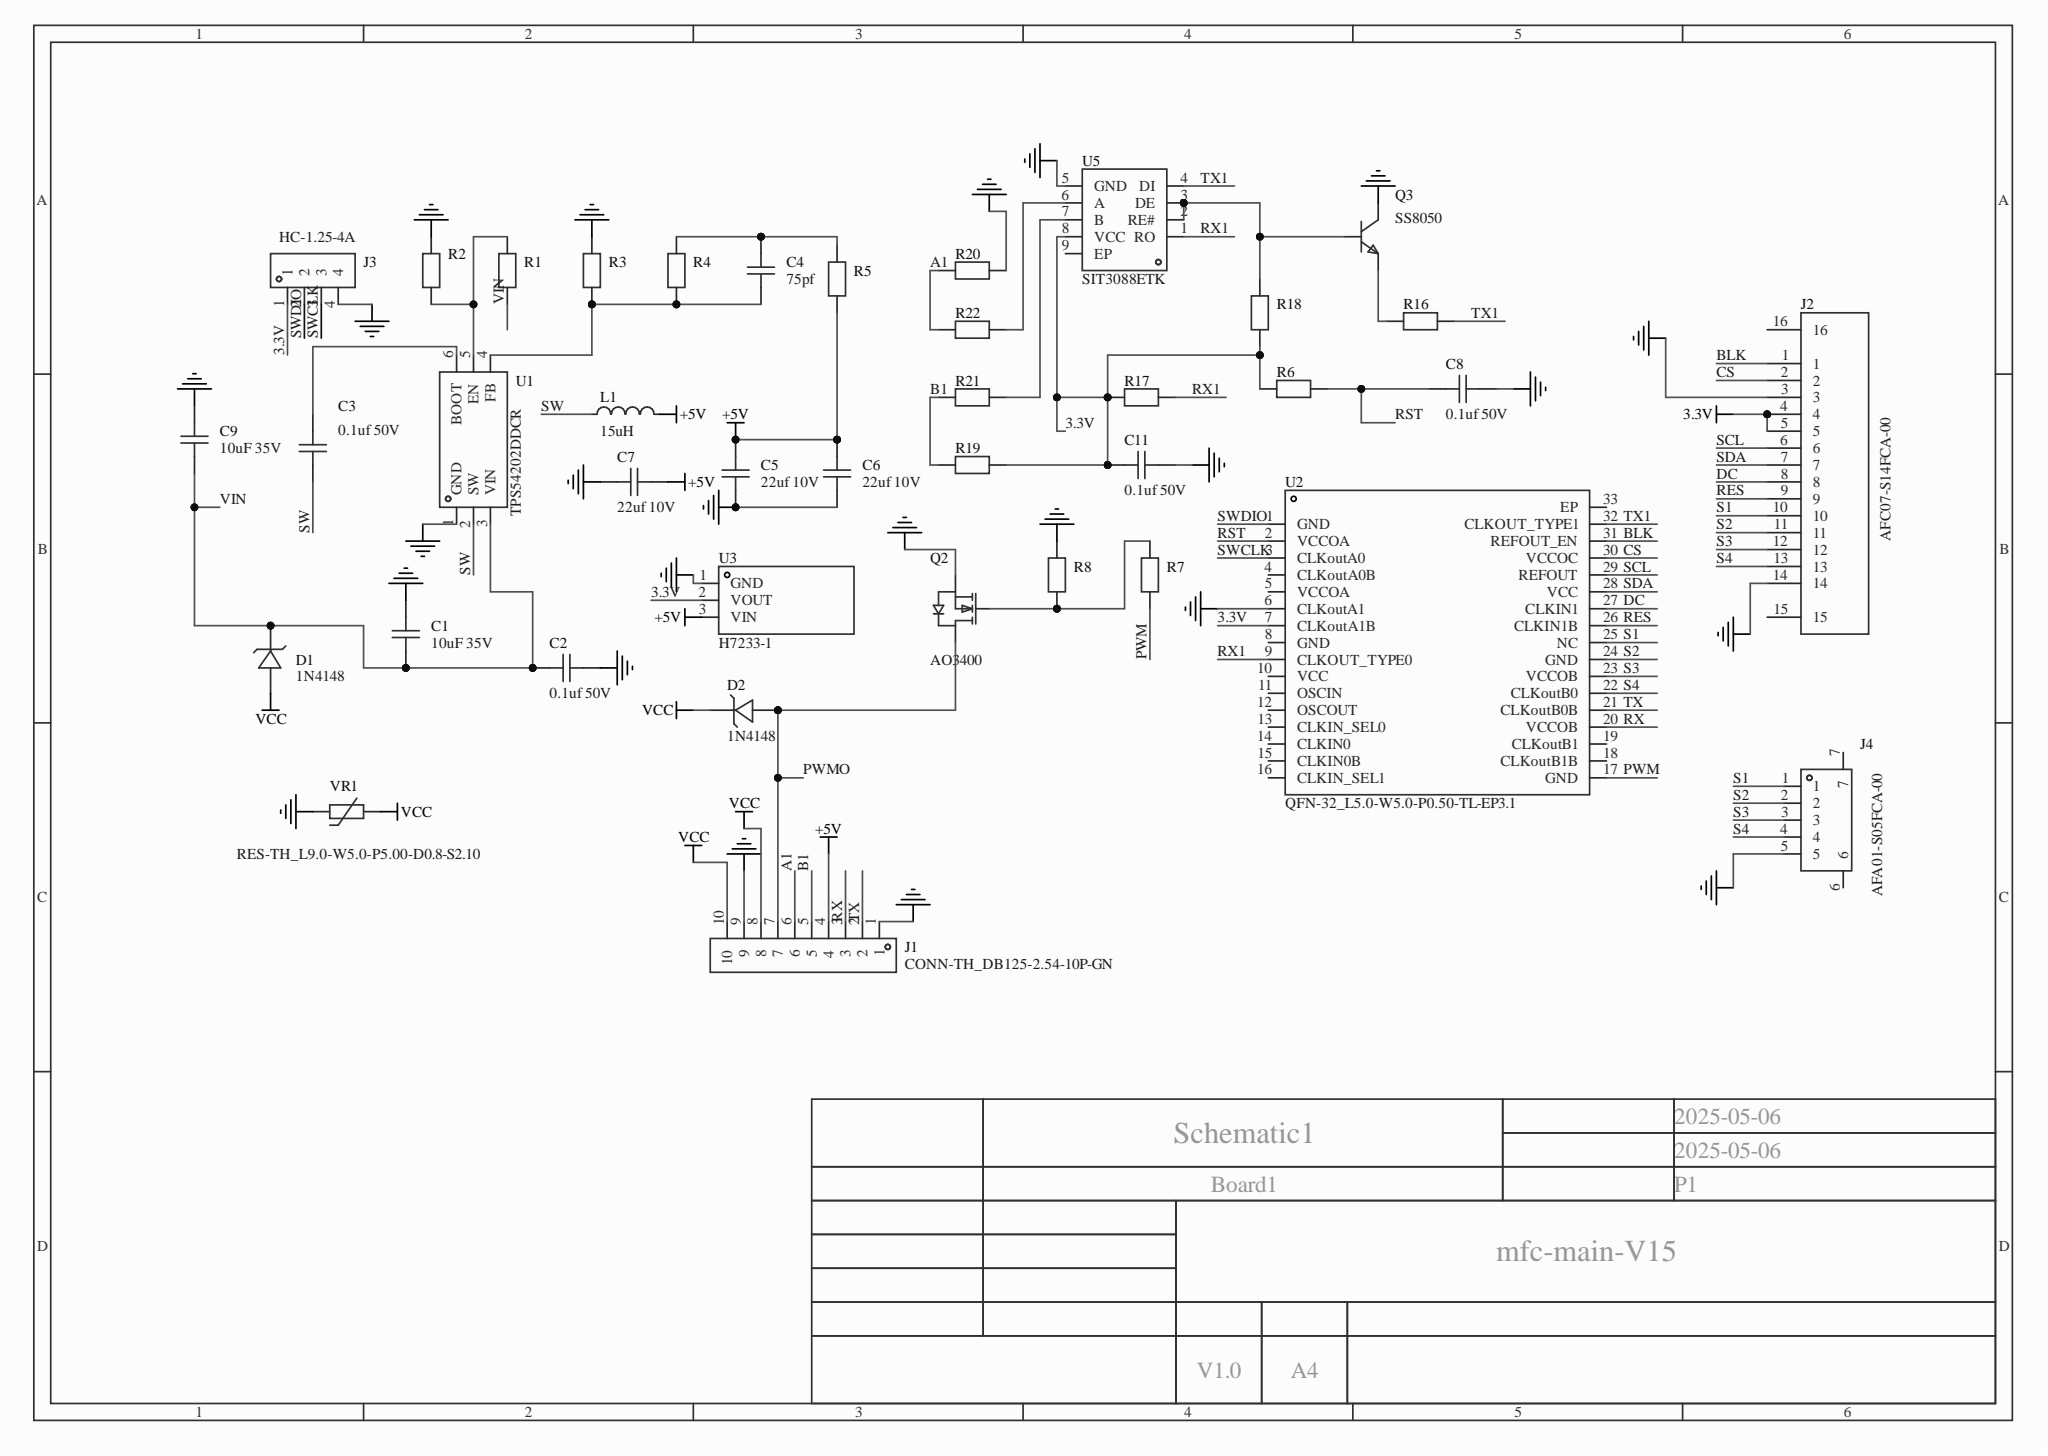Circuit board | Altium Designer | 39 parts | 36 nets
Bill of materials:
Comment,Description,Designator,Footprint,LibRef,Quantity
"10uF 35V","","C1, C9","C0805","CL21A106KAYNNNE_C15850","2"
"0.1uf 50V","","C2, C3, C8, C11","C0603","CT41-0603-2F4-50V-0.1uF-M(N)","4"
"75pf","","C4","C0603","CT41-0603-2F4-50V-0.1uF-M(N)","1"
"22uf 10V","","C5, C6, C7","C0603","CT41-0603-2F4-50V-0.1uF-M(N)","3"
"1N4148","","D1, D2","SOD-123_L2.7-W1.7-LS3.8-RD","1N4148","2"
"CONN-TH_DB125-2.54-10P-GN","","J1","CONN-TH_DB125-2.54-10P-GN","DB125-2.54-10P-GN-S","1"
"AFC07-S14FCA-00","","J2","FPC-SMD_14P-P0.50_AFC07-S14FCA-00","AFC07-S14FCA-00","1"
"HC-1.25-4A","","J3","CONN-TH_4P-P1.25_HCTL_HC-1.25-4A","HC-1.25-4A","1"
"AFA01-S05FCA-00","","J4","FPC-SMD_AFA01-S05FCA-00","AFA01-S05FCA-00","1"
"15uH","","L1","IND-SMD_L3.5-W3.0","CMLF0302-150MTT","1"
"AO3400","","Q2","SOT-23-3_L2.9-W1.3-P1.90-LS2.4-BL-2","AO3400","1"
"SS8050","","Q3","SOT-23-3_L2.9-W1.3-P1.90-LS2.4-BR","SS8050","1"
"","","R1, R2, R3, R4, R5, R6, R7, R8, R16, R17, R18, R19, R20, R21, R22","R0603","RT0603BRD07105KL","15"
"TPS54202DDCR","","U1","SOT-23-6_L2.9-W1.6-P0.95-LS2.8-BL","TPS54202DDCR","1"
"QFN-32_L5.0-W5.0-P0.50-TL-EP3.1","","U2","QFN-32_L5.0-W5.0-P0.50-TL-EP3.1","NCS25D34","1"
"H7233-1","","U3","SOT-23-3_L2.9-W1.3-P1.90-LS2.4-BR","H7233-1","1"
"SIT3088ETK","","U5","DFN-8_L3.0-W3.0-P0.65-BL-EP","SIT3088ETK","1"
"RES-TH_L9.0-W5.0-P5.00-D0.8-S2.10","","VR1","RES-TH_L9.0-W5.0-P5.00-D0.8-S2.10","FTR07D390K","1"
Netlist (Protel format):
[
C1
C0805
10uF 35V



]
[
C2
C0603
0.1uf 50V



]
[
C3
C0603
0.1uf 50V



]
[
C4
C0603
75pf



]
[
C5
C0603
22uf 10V



]
[
C6
C0603
22uf 10V



]
[
C7
C0603
22uf 10V



]
[
C8
C0603
0.1uf 50V



]
[
C9
C0805
10uF 35V



]
[
C11
C0603
0.1uf 50V



]
[
D1
SOD-123_L2.7-W1.7-LS3.8-RD
1N4148



]
[
D2
SOD-123_L2.7-W1.7-LS3.8-RD
1N4148



]
[
J1
CONN-TH_DB125-2.54-10P-GN
CONN-TH_DB125-2.54-10P-GN



]
[
J2
FPC-SMD_14P-P0.50_AFC07-S14FCA-00
AFC07-S14FCA-00



]
[
J3
CONN-TH_4P-P1.25_HCTL_HC-1.25-4A
HC-1.25-4A



]
[
J4
FPC-SMD_AFA01-S05FCA-00
AFA01-S05FCA-00



]
[
L1
IND-SMD_L3.5-W3.0
15uH



]
[
Q2
SOT-23-3_L2.9-W1.3-P1.90-LS2.4-BL-2
AO3400



]
[
Q3
SOT-23-3_L2.9-W1.3-P1.90-LS2.4-BR
SS8050



]
[
R1
R0603




]
[
R2
R0603




]
[
R3
R0603




]
[
R4
R0603




]
[
R5
R0603




]
[
R6
R0603




]
[
R7
R0603




]
[
R8
R0603




]
[
R16
R0603




]
[
R17
R0603




]
[
R18
R0603




]
[
R19
R0603




]
[
R20
R0603




]
[
R21
R0603




]
[
R22
R0603




]
[
U1
SOT-23-6_L2.9-W1.6-P0.95-LS2.8-BL
TPS54202DDCR



]
[
U2
QFN-32_L5.0-W5.0-P0.50-TL-EP3.1
QFN-32_L5.0-W5.0-P0.50-TL-EP3.1



]
[
U3
SOT-23-3_L2.9-W1.3-P1.90-LS2.4-BR
H7233-1



]
[
U5
DFN-8_L3.0-W3.0-P0.65-BL-EP
SIT3088ETK



]
[
VR1
RES-TH_L9.0-W5.0-P5.00-D0.8-S2.10
RES-TH_L9.0-W5.0-P5.00-D0.8-S2.10



]
(
VIN
C1-1
C2-2
C9-1
D1-1
R1-1
U1-3
)
(
VCC
D1-2
D2-1
J1-8
J1-10
VR1-2
)
(
TX1
R16-2
U2-32
U5-4
)
(
TX
J1-2
U2-21
)
(
SWDIO
J3-2
U2-1
)
(
SWCLK
J3-3
U2-3
)
(
SW
C3-1
L1-1
U1-2
)
(
SDA
J2-7
U2-28
)
(
SCL
J2-6
U2-29
)
(
S4
J2-13
J4-4
U2-22
)
(
S3
J2-12
J4-3
U2-23
)
(
S2
J2-11
J4-2
U2-24
)
(
S1
J2-10
J4-1
U2-25
)
(
RX1
R17-2
U2-9
U5-1
)
(
RX
J1-3
U2-20
)
(
RST
C8-2
R6-2
U2-2
)
(
RES
J2-9
U2-26
)
(
PWMO
D2-2
J1-7
Q2-3
)
(
PWM
R7-1
U2-17
)
(
NetR22_2
R22-2
U5-6
)
(
NetR21_2
R21-2
U5-7
)
(
NetR1_2
R1-2
R2-1
U1-5
)
(
NetQ3_2
Q3-2
R16-1
)
(
NetQ3_1
Q3-1
R18-2
U5-2
U5-3
)
(
NetQ2_1
Q2-1
R7-2
R8-1
)
(
NetC4_2
C4-2
R3-1
R4-1
U1-4
)
(
NetC4_1
C4-1
R4-2
R5-2
)
(
NetC3_2
C3-2
U1-6
)
(
GND
C1-2
C2-1
C5-2
C6-2
C7-2
C8-1
C9-2
C11-1
J1-1
J1-9
J2-3
J2-14
J3-4
J4-5
Q2-2
Q3-3
R2-2
R3-2
R8-2
R20-2
U1-1
U2-6
U3-1
U5-5
VR1-1
)
(
DC
J2-8
U2-27
)
(
CS
J2-2
U2-30
)
(
BLK
J2-1
U2-31
)
(
B1
J1-5
R19-1
R21-1
)
(
A1
J1-6
R20-1
R22-1
)
(
+5V
C5-1
C6-1
C7-1
J1-4
L1-2
R5-1
U3-3
)
(
3.3V
C11-2
J2-4
J2-5
J3-1
R6-1
R17-1
R18-1
R19-2
U2-7
U3-2
U5-8
)